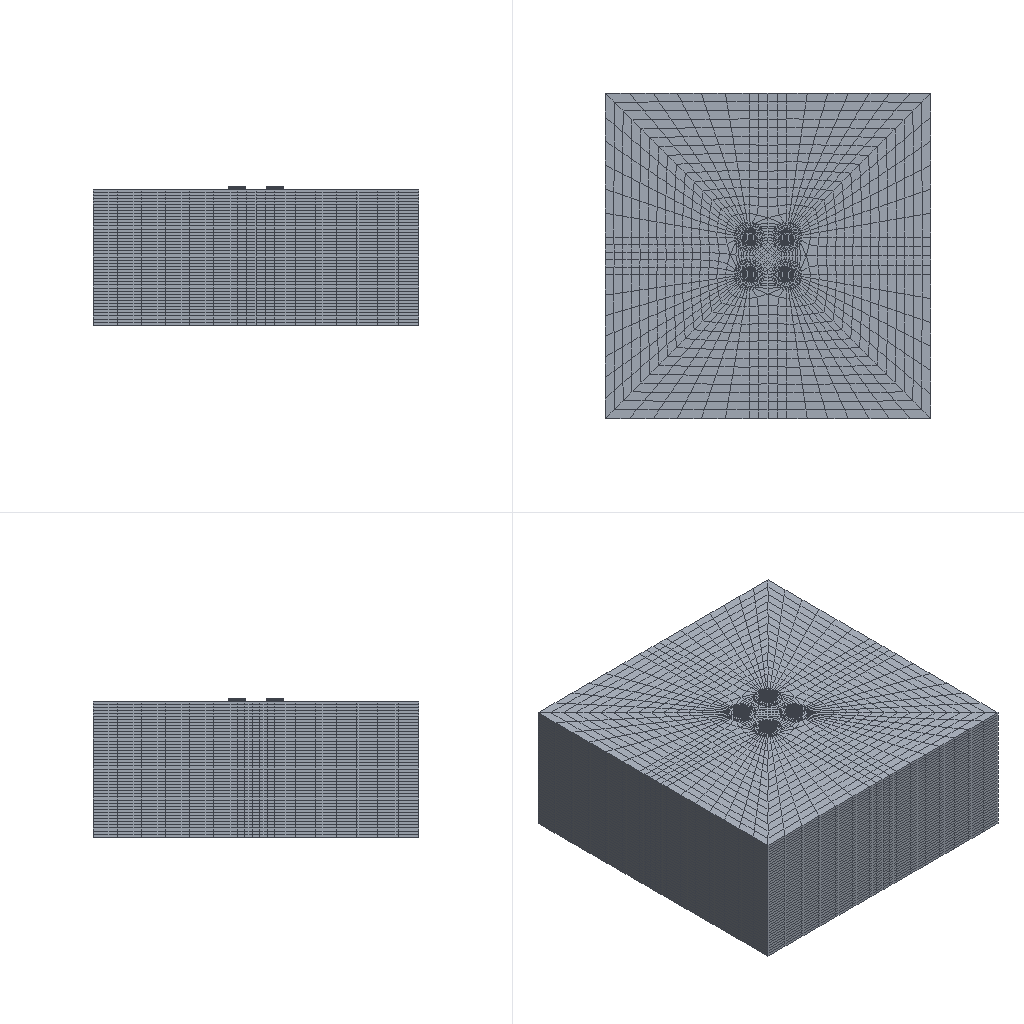Simulation study | abaqus
Set-up summary:
category,name,step,type,value,unit,region
solver,abaqus
solver,version,,,Abaqus/Standard 2020
units,not stated in the deck,,not stated
analysis,deck,,static,static
load_step,Step-digit-1,Step-digit-1,static
load_step,requested,,,1
mesh,nodes,,,107772
mesh,elements,,,93262
element_type,B31,,beam,40
element_type,C3D10,,solid,3792
element_type,C3D8R,,solid,89430
load,load commands in deck,,count,1
bc,support commands in deck,,count,3
material,TIE,,in results
material,TUTI,,in results
check,setup vs results,,match,"per instance, exact: element labels, types and connectivity; labels of the nodes the elements use; coordinates of those nodes at SINGLE_PRECISION in 8 of 21 instance(s)"
Abaqus input file, long lists of numbers shortened, first 379 of 1982 lines:
*Heading
** Job name: Job-1 Model name: Model-1
** Generated by: Abaqus/CAE 2020
*Preprint, echo=NO, model=NO, history=NO, contact=NO
**
** PARTS
**
*Part, name=chongshuatu
*Node
      1,           0., -0.0546, -0.1365
      2,           0.,           0., -0.1365
** (1960 more lines like these left out)
*Element, type=C3D10
  1, 321, 151,  35,  33, 350, 349, 348, 352, 351, 353
  2, 321, 152,  23,  34, 356, 355, 354, 358, 357, 359
** (946 more lines like these left out)
*Nset, nset=Set-chongshuatu, generate
    1,  1962,     1
*Elset, elset=Set-chongshuatu, generate
   1,  948,    1
** Section: Section-tuti
*Solid Section, elset=Set-chongshuatu, material=tuti
,
*End Part
**
*Part, name=daoguanzu
*Node
      1,           0.,           0.,           0.
      2,           0., 0.005,           0.
** (9 more lines like these left out)
*Element, type=B31
 1,  1,  2
 2,  2,  3
** (8 more lines like these left out)
*Nset, nset=Set-dgjzu, generate
  1,  11,   1
*Elset, elset=Set-dgjzu, generate
  1,  10,   1
** Section: Section-daoguanjia  Profile: Profile-dgj
*Beam Section, elset=Set-dgjzu, material=tie, temperature=GRADIENTS, section=CIRC
0.01
0.,0.,-1.
*End Part
**
*Part, name=tonggai
*Node
      1,  0.1365,           0.,           0.
      2,           0.,           0.,           0.
** (691 more lines like these left out)
*Element, type=C3D8R
  1, 194, 195, 545, 540,  15,  16, 149, 148
  2, 195, 196, 546, 545,  16,  17, 150, 149
** (414 more lines like these left out)
*Nset, nset=Set-tonggai, generate
   1,  693,    1
*Elset, elset=Set-tonggai, generate
   1,  416,    1
** Section: Section-tong
*Solid Section, elset=Set-tonggai, material=tie
,
*End Part
**
*Part, name=tongneitu
*Node
      1,  0.1265,           0.,           0.
      2,           0.,           0.,           0.
** (1307 more lines like these left out)
*Element, type=C3D8R
  1, 194, 195, 736, 680,  13,  14, 141, 140
  2, 195, 196, 737, 736,  14,  15, 142, 141
** (1038 more lines like these left out)
*Nset, nset=Set-tongneitu, generate
    1,  1309,     1
*Elset, elset=Set-tongneitu, generate
    1,  1040,     1
** Section: Section-tuti
*Solid Section, elset=Set-tongneitu, material=tuti
,
*End Part
**
*Part, name=tongqun
*Node
      1,           0.,  0.1265,  0.273
      2,           0.,  0.1265,           0.
** (2126 more lines like these left out)
*Element, type=C3D8R
  1,    8,  113,  752,  158,    1,    9,  293,   96
  2,  113,  112,  753,  752,    9,   10,  294,  293
** (1006 more lines like these left out)
*Nset, nset=Set-tongqun, generate
    1,  2128,     1
*Elset, elset=Set-tongqun, generate
    1,  1008,     1
** Section: Section-tong
*Solid Section, elset=Set-tongqun, material=tie
,
*End Part
**
*Part, name=tuti
*Node
      1,  -2.827,   2.417,  -2.184
      2,  -2.924,    2.32,  -2.184
** (83358 more lines like these left out)
*Element, type=C3D8R
  1,  4702,  4703, 33021, 32910,   204,   205,  4621,  4620
  2,  4703,  4704, 33022, 33021,   205,   206,  4622,  4621
** (79572 more lines like these left out)
*Nset, nset=Set-tuti, generate
     1,  83360,      1
*Elset, elset=Set-tuti, generate
     1,  79574,      1
** Section: Section-tuti
*Solid Section, elset=Set-tuti, material=tuti
,
*End Part
**
**
** ASSEMBLY
**
*Assembly, name=Assembly
**
*Instance, name=tonggai-1, part=tonggai
      0.3015,      -0.3015,         0.04
*End Instance
**
*Instance, name=tongneitu-1, part=tongneitu
      0.3015,      -0.3015,       -0.233
*End Instance
**
*Instance, name=tongqun-1, part=tongqun
      0.3015,      -0.3015,       -0.233
*End Instance
**
*Instance, name=tuti-1, part=tuti
       2.622,       -2.622,           0.
*End Instance
**
*Instance, name=tonggai-1-lin-1-2, part=tonggai
      0.3015,       0.3015,         0.04
*End Instance
**
*Instance, name=tonggai-1-lin-2-1, part=tonggai
     -0.3015,      -0.3015,         0.04
*End Instance
**
*Instance, name=tonggai-1-lin-2-2, part=tonggai
     -0.3015,       0.3015,         0.04
*End Instance
**
*Instance, name=tongneitu-1-lin-1-2, part=tongneitu
      0.3015,       0.3015,       -0.233
*End Instance
**
*Instance, name=tongneitu-1-lin-2-1, part=tongneitu
     -0.3015,      -0.3015,       -0.233
*End Instance
**
*Instance, name=tongneitu-1-lin-2-2, part=tongneitu
     -0.3015,       0.3015,       -0.233
*End Instance
**
*Instance, name=tongqun-1-lin-1-2, part=tongqun
      0.3015,       0.3015,       -0.233
*End Instance
**
*Instance, name=tongqun-1-lin-2-1, part=tongqun
     -0.3015,      -0.3015,       -0.233
*End Instance
**
*Instance, name=tongqun-1-lin-2-2, part=tongqun
     -0.3015,       0.3015,       -0.233
*End Instance
**
*Instance, name=chongshuatu-1, part=chongshuatu
      0.3015,      -0.3015,           0.
      0.3015,      -0.3015,           0., 1.302,      -0.3015,           0., 90.
*End Instance
**
*Instance, name=chongshuatu-1-lin-1-2, part=chongshuatu
      0.3015,       0.3015,           0.
      0.3015,       0.3015,           0., 1.302,       0.3015,           0., 90.
*End Instance
**
*Instance, name=chongshuatu-1-lin-2-1, part=chongshuatu
     -0.3015,      -0.3015,           0.
     -0.3015,      -0.3015,           0., 0.6985,      -0.3015,           0., 90.
*End Instance
**
*Instance, name=chongshuatu-1-lin-2-2, part=chongshuatu
     -0.3015,       0.3015,           0.
     -0.3015,       0.3015,           0., 0.6985,       0.3015,           0., 90.
*End Instance
**
*Instance, name=daoguanzu-1, part=daoguanzu
     -0.3015,      -0.3015,         0.05
     -0.3015,      -0.3015,         0.05, 0.6985,      -0.3015,         0.05, 90.
*End Instance
**
*Instance, name=daoguanzu-1-lin-1-2, part=daoguanzu
     -0.3015,       0.3015,         0.05
     -0.3015,       0.3015,         0.05, 0.6985,       0.3015,         0.05, 90.
*End Instance
**
*Instance, name=daoguanzu-1-lin-2-1, part=daoguanzu
0.3015,      -0.3015,         0.05
0.3015,      -0.3015,         0.05, 1.302,      -0.3015,         0.05, 90.
*End Instance
**
*Instance, name=daoguanzu-1-lin-2-2, part=daoguanzu
0.3015,       0.3015,         0.05
0.3015,       0.3015,         0.05, 1.302,       0.3015,         0.05, 90.
*End Instance
**
*Nset, nset=Set-10, instance=chongshuatu-1, generate
    1,  1962,     1
*Elset, elset=Set-10, instance=chongshuatu-1, generate
   1,  948,    1
*Nset, nset=Set-11, instance=chongshuatu-1-lin-1-2, generate
    1,  1962,     1
*Elset, elset=Set-11, instance=chongshuatu-1-lin-1-2, generate
   1,  948,    1
*Nset, nset=Set-12, instance=chongshuatu-1-lin-2-2, generate
    1,  1962,     1
*Elset, elset=Set-12, instance=chongshuatu-1-lin-2-2, generate
   1,  948,    1
*Nset, nset=Set-13, instance=chongshuatu-1-lin-2-1, generate
    1,  1962,     1
*Elset, elset=Set-13, instance=chongshuatu-1-lin-2-1, generate
   1,  948,    1
*Nset, nset=Set-14, instance=tuti-1
     1,     2,     3,    10,    11,    12,    25,    26,    27,    28,    31,    32,    35,    36,    44,    45
    46,    47,    48,    49,    50,    51,    52,    63,    64,    65,    81,    82,    83,    84,    88,    91
** (117 more lines like these left out)
*Elset, elset=Set-14, instance=tuti-1
     1,     2,     3,     4,     5,     6,   115,   116,   117,   172,   173,   734,   735,   774,   775,   814
   815,   873,   893,   913,   933,   953,   973,   974,   975,  1014,  1015,  5569,  5570,  5571,  5572,  5573
** (114 more lines like these left out)
*Nset, nset=Set-15, instance=tuti-1
    13,    16,    17,    20,    22,    25,    47,    48,    85,   113,   120,   141,   154,   155,   156,   157
   159,   160,   162,   163,   166,   167,   168,   183,   506,   507,   508,   509,   510,   511,   546,   547
** (100 more lines like these left out)
*Elset, elset=Set-15, instance=tuti-1
  1054,  1069,  1084,  1099,  1114,  1129,  1144,  1159,  1174,  1189,  1204,  1219,  1234,  1249,  1264,  1279
  1294,  1309,  1324,  1339,  1354,  1369,  1384,  1399,  1414,  1429,  1444,  1459,  1474,  1489,  1504,  1519
** (92 more lines like these left out)
*Nset, nset=Set-16, instance=tuti-1
    13,    17,    22,    23,    25,    26,    47,    85,    86,   113,   116,   119,   120,   141,   144,   154
   157,   159,   177,   178,   179,   198,   199,   202,   556,   557,   558,   559,   582,   583,   584,   585
** (100 more lines like these left out)
*Elset, elset=Set-16, instance=tuti-1
  1593,  1608,  1623,  1638,  1653,  1668,  1683,  1698,  1713,  1728,  1743,  1758,  1773,  1788,  1803,  1818
  1833,  1848,  1863,  1878,  1893,  1908,  1923,  1938,  1953,  1968,  1983,  1998,  2013,  2028,  2043,  2058
** (92 more lines like these left out)
*Nset, nset=Set-di, instance=tuti-1
     1,     2,     3,    10,    11,    12,    25,    26,    27,    28,    31,    32,    35,    36,    44,    45
    46,    47,    48,    49,    50,    51,    52,    63,    64,    65,    81,    82,    83,    84,    88,    91
** (117 more lines like these left out)
*Elset, elset=Set-di, instance=tuti-1
     1,     2,     3,     4,     5,     6,   115,   116,   117,   172,   173,   734,   735,   774,   775,   814
   815,   873,   893,   913,   933,   953,   973,   974,   975,  1014,  1015,  5569,  5570,  5571,  5572,  5573
** (114 more lines like these left out)
*Nset, nset=Set-shuiping, instance=tuti-1
    13,    16,    17,    20,    22,    23,    25,    26,    47,    48,    85,    86,   113,   116,   119,   120
   141,   144,   154,   155,   156,   157,   159,   160,   162,   163,   166,   167,   168,   177,   178,   179
** (190 more lines like these left out)
*Elset, elset=Set-shuiping, instance=tuti-1
  1054,  1069,  1084,  1099,  1114,  1129,  1144,  1159,  1174,  1189,  1204,  1219,  1234,  1249,  1264,  1279
  1294,  1309,  1324,  1339,  1354,  1369,  1384,  1399,  1414,  1429,  1444,  1459,  1474,  1489,  1504,  1519
** (185 more lines like these left out)
*Nset, nset=b_Set-5, instance=tonggai-1, generate
   1,  693,    1
*Nset, nset=b_Set-5, instance=tongqun-1, generate
    1,  2128,     1
*Nset, nset=b_Set-5, instance=tonggai-1-lin-1-2, generate
   1,  693,    1
*Nset, nset=b_Set-5, instance=tonggai-1-lin-2-2, generate
   1,  693,    1
*Nset, nset=b_Set-5, instance=tongqun-1-lin-1-2, generate
    1,  2128,     1
*Nset, nset=b_Set-5, instance=daoguanzu-1, generate
  1,  11,   1
*Nset, nset=b_Set-5, instance=tongqun-1-lin-2-2, generate
    1,  2128,     1
*Nset, nset=b_Set-5, instance=daoguanzu-1-lin-2-1, generate
  1,  11,   1
*Nset, nset=b_Set-5, instance=tonggai-1-lin-2-1, generate
   1,  693,    1
*Nset, nset=b_Set-5, instance=tongqun-1-lin-2-1, generate
    1,  2128,     1
*Nset, nset=b_Set-5, instance=daoguanzu-1-lin-1-2, generate
  1,  11,   1
*Nset, nset=b_Set-5, instance=daoguanzu-1-lin-2-2, generate
  1,  11,   1
*Elset, elset=b_Set-5, instance=tonggai-1, generate
   1,  416,    1
*Elset, elset=b_Set-5, instance=tongqun-1, generate
    1,  1008,     1
*Elset, elset=b_Set-5, instance=tonggai-1-lin-1-2, generate
   1,  416,    1
*Elset, elset=b_Set-5, instance=tonggai-1-lin-2-2, generate
   1,  416,    1
*Elset, elset=b_Set-5, instance=tongqun-1-lin-1-2, generate
    1,  1008,     1
*Elset, elset=b_Set-5, instance=daoguanzu-1, generate
  1,  10,   1
*Elset, elset=b_Set-5, instance=tongqun-1-lin-2-2, generate
    1,  1008,     1
*Elset, elset=b_Set-5, instance=daoguanzu-1-lin-2-1, generate
  1,  10,   1
*Elset, elset=b_Set-5, instance=tonggai-1-lin-2-1, generate
   1,  416,    1
*Elset, elset=b_Set-5, instance=tongqun-1-lin-2-1, generate
    1,  1008,     1
*Elset, elset=b_Set-5, instance=daoguanzu-1-lin-1-2, generate
  1,  10,   1
*Elset, elset=b_Set-5, instance=daoguanzu-1-lin-2-2, generate
  1,  10,   1
*Nset, nset=b_Set-6, instance=tonggai-1, generate
   1,  693,    1
*Nset, nset=b_Set-6, instance=tongqun-1, generate
    1,  2128,     1
*Nset, nset=b_Set-6, instance=tonggai-1-lin-1-2, generate
   1,  693,    1
*Nset, nset=b_Set-6, instance=tonggai-1-lin-2-2, generate
   1,  693,    1
*Nset, nset=b_Set-6, instance=tongqun-1-lin-1-2, generate
    1,  2128,     1
*Nset, nset=b_Set-6, instance=daoguanzu-1, generate
  1,  11,   1
*Nset, nset=b_Set-6, instance=tongqun-1-lin-2-2, generate
    1,  2128,     1
*Nset, nset=b_Set-6, instance=daoguanzu-1-lin-2-1, generate
  1,  11,   1
*Nset, nset=b_Set-6, instance=tonggai-1-lin-2-1, generate
   1,  693,    1
*Nset, nset=b_Set-6, instance=tongqun-1-lin-2-1, generate
    1,  2128,     1
*Nset, nset=b_Set-6, instance=daoguanzu-1-lin-1-2, generate
  1,  11,   1
*Nset, nset=b_Set-6, instance=daoguanzu-1-lin-2-2, generate
  1,  11,   1
*Elset, elset=b_Set-6, instance=tonggai-1, generate
   1,  416,    1
*Elset, elset=b_Set-6, instance=tongqun-1, generate
    1,  1008,     1
*Elset, elset=b_Set-6, instance=tonggai-1-lin-1-2, generate
   1,  416,    1
*Elset, elset=b_Set-6, instance=tonggai-1-lin-2-2, generate
   1,  416,    1
*Elset, elset=b_Set-6, instance=tongqun-1-lin-1-2, generate
    1,  1008,     1
*Elset, elset=b_Set-6, instance=daoguanzu-1, generate
  1,  10,   1
*Elset, elset=b_Set-6, instance=tongqun-1-lin-2-2, generate
    1,  1008,     1
*Elset, elset=b_Set-6, instance=daoguanzu-1-lin-2-1, generate
  1,  10,   1
*Elset, elset=b_Set-6, instance=tonggai-1-lin-2-1, generate
   1,  416,    1
*Elset, elset=b_Set-6, instance=tongqun-1-lin-2-1, generate
    1,  1008,     1
*Elset, elset=b_Set-6, instance=daoguanzu-1-lin-1-2, generate
  1,  10,   1
*Elset, elset=b_Set-6, instance=daoguanzu-1-lin-2-2, generate
  1,  10,   1
*Nset, nset=s_Set-zu1, instance=daoguanzu-1-lin-1-2
 1,
*Nset, nset=s_Set-zu2, instance=daoguanzu-1-lin-2-2
 1,
*Nset, nset=s_Set-zu3, instance=daoguanzu-1-lin-2-1
 1,
*Nset, nset=s_Set-zu4, instance=daoguanzu-1
 1,
*Elset, elset=_Surf-tongdi1_S6, internal, instance=tongqun-1-lin-2-2, generate
 505,  991,   18
*Elset, elset=_Surf-tongdi1_S4, internal, instance=tongqun-1-lin-2-2, generate
  18,  504,   18
*Surface, type=ELEMENT, name=Surf-tongdi1
_Surf-tongdi1_S6, S6
Last 618 lines:
*Surface, type=ELEMENT, name=_Int-1_gcs0_535, internal
__Int-1_gcs0_535_S3, S3
__Int-1_gcs0_535_S4, S4
*Elset, elset=__Int-1_gcs0_536_S4, internal, instance=tongneitu-1-lin-2-2
  842,  844,  846,  848,  850,  852,  854,  856,  858,  860,  862,  864,  866,  868,  870,  872
  874,  876,  878,  880,  912,  914,  916,  918,  920,  922,  924,  926,  928,  930,  932,  934
** (2 more lines like these left out)
*Elset, elset=__Int-1_gcs0_536_S3, internal, instance=tongneitu-1-lin-2-2
 881, 882, 883, 887, 888, 889, 893, 894, 895, 899, 900, 901, 905, 906, 907
*Surface, type=ELEMENT, name=_Int-1_gcs0_536, internal
__Int-1_gcs0_536_S4, S4
__Int-1_gcs0_536_S3, S3
*Elset, elset=__Int-1_gcs0_542_S1, internal, instance=tongqun-1-lin-1-2, generate
  505,  1008,     1
*Surface, type=ELEMENT, name=_Int-1_gcs0_542, internal
__Int-1_gcs0_542_S1, S1
*Elset, elset=__Int-1_gcs0_544_S2, internal, instance=tongqun-1-lin-1-2, generate
   1,  504,    1
*Surface, type=ELEMENT, name=_Int-1_gcs0_544, internal
__Int-1_gcs0_544_S2, S2
*Elset, elset=__Int-1_gcs0_545_S1, internal, instance=tongqun-1-lin-1-2, generate
   1,  504,    1
*Surface, type=ELEMENT, name=_Int-1_gcs0_545, internal
__Int-1_gcs0_545_S1, S1
*Elset, elset=__Int-1_gcs0_546_S2, internal, instance=tongqun-1-lin-1-2, generate
  505,  1008,     1
*Surface, type=ELEMENT, name=_Int-1_gcs0_546, internal
__Int-1_gcs0_546_S2, S2
*Elset, elset=__Int-1_gcs0_552_S1, internal, instance=tongqun-1-lin-2-1, generate
  505,  1008,     1
*Surface, type=ELEMENT, name=_Int-1_gcs0_552, internal
__Int-1_gcs0_552_S1, S1
*Elset, elset=__Int-1_gcs0_554_S2, internal, instance=tongqun-1-lin-2-1, generate
   1,  504,    1
*Surface, type=ELEMENT, name=_Int-1_gcs0_554, internal
__Int-1_gcs0_554_S2, S2
*Elset, elset=__Int-1_gcs0_555_S1, internal, instance=tongqun-1-lin-2-1, generate
   1,  504,    1
*Surface, type=ELEMENT, name=_Int-1_gcs0_555, internal
__Int-1_gcs0_555_S1, S1
*Elset, elset=__Int-1_gcs0_556_S2, internal, instance=tongqun-1-lin-2-1, generate
  505,  1008,     1
*Surface, type=ELEMENT, name=_Int-1_gcs0_556, internal
__Int-1_gcs0_556_S2, S2
*Elset, elset=__Int-1_gcs0_562_S1, internal, instance=tongqun-1-lin-2-2, generate
  505,  1008,     1
*Surface, type=ELEMENT, name=_Int-1_gcs0_562, internal
__Int-1_gcs0_562_S1, S1
*Elset, elset=__Int-1_gcs0_564_S2, internal, instance=tongqun-1-lin-2-2, generate
   1,  504,    1
*Surface, type=ELEMENT, name=_Int-1_gcs0_564, internal
__Int-1_gcs0_564_S2, S2
*Elset, elset=__Int-1_gcs0_565_S1, internal, instance=tongqun-1-lin-2-2, generate
   1,  504,    1
*Surface, type=ELEMENT, name=_Int-1_gcs0_565, internal
__Int-1_gcs0_565_S1, S1
*Elset, elset=__Int-1_gcs0_566_S2, internal, instance=tongqun-1-lin-2-2, generate
  505,  1008,     1
*Surface, type=ELEMENT, name=_Int-1_gcs0_566, internal
__Int-1_gcs0_566_S2, S2
*Elset, elset=__Int-1_gcs0_572_S3, internal, instance=chongshuatu-1
  16,  23,  45,  51,  72,  80,  84,  96,  98,  99, 101, 102, 106, 111, 116, 130
 134, 139, 141, 142, 145, 149, 165, 173, 178, 183, 190, 194, 218, 243
*Elset, elset=__Int-1_gcs0_572_S4, internal, instance=chongshuatu-1
  33,  90, 112, 120, 132, 174, 175, 185, 209, 213, 216, 226
*Elset, elset=__Int-1_gcs0_572_S1, internal, instance=chongshuatu-1
  78,  83,  95, 128, 136, 147, 168, 179, 182, 187, 204, 206, 210, 228, 233, 240
 242,
*Elset, elset=__Int-1_gcs0_572_S2, internal, instance=chongshuatu-1
  81,  89, 191, 207, 238
*Surface, type=ELEMENT, name=_Int-1_gcs0_572, internal
__Int-1_gcs0_572_S3, S3
__Int-1_gcs0_572_S4, S4
__Int-1_gcs0_572_S2, S2
__Int-1_gcs0_572_S1, S1
*Elset, elset=__Int-1_gcs0_573_S3, internal, instance=chongshuatu-1
  61, 148, 153, 160, 169, 170, 171, 172, 175, 179, 180, 181, 182, 184, 187, 188
 189, 191, 192, 193, 199, 200, 203, 205, 207, 210, 211, 217, 238
*Elset, elset=__Int-1_gcs0_573_S1, internal, instance=chongshuatu-1
  94, 151
*Elset, elset=__Int-1_gcs0_573_S2, internal, instance=chongshuatu-1
 186,
*Surface, type=ELEMENT, name=_Int-1_gcs0_573, internal
__Int-1_gcs0_573_S3, S3
__Int-1_gcs0_573_S1, S1
__Int-1_gcs0_573_S2, S2
*Elset, elset=__Int-1_gcs0_574_S3, internal, instance=chongshuatu-1
 534, 543, 593, 634, 642, 645, 652, 658, 661, 662, 670, 674, 675, 676, 680, 681
 682, 685, 690, 692, 694, 697, 698, 703, 706, 707, 708, 716, 718, 727
*Elset, elset=__Int-1_gcs0_574_S2, internal, instance=chongshuatu-1
 663,
*Elset, elset=__Int-1_gcs0_574_S4, internal, instance=chongshuatu-1
 664,
*Surface, type=ELEMENT, name=_Int-1_gcs0_574, internal
__Int-1_gcs0_574_S3, S3
__Int-1_gcs0_574_S2, S2
__Int-1_gcs0_574_S4, S4
*Elset, elset=__Int-1_gcs0_575_S3, internal, instance=chongshuatu-1
 252, 283, 306, 312, 315, 321, 337, 363, 366, 367, 374, 389, 416, 429, 434, 444
 458, 465, 469, 479
*Elset, elset=__Int-1_gcs0_575_S2, internal, instance=chongshuatu-1
 269, 314, 328, 377, 384, 412, 446, 448
*Elset, elset=__Int-1_gcs0_575_S1, internal, instance=chongshuatu-1
 308, 309, 313, 318, 323, 332, 339, 342, 346, 347, 348, 378, 380, 400, 415, 420
 431, 450, 453, 466, 489
*Elset, elset=__Int-1_gcs0_575_S4, internal, instance=chongshuatu-1
 310, 311, 319, 331, 344, 355, 357, 358, 361, 369, 371, 382, 394, 402, 433
*Surface, type=ELEMENT, name=_Int-1_gcs0_575, internal
__Int-1_gcs0_575_S3, S3
__Int-1_gcs0_575_S2, S2
__Int-1_gcs0_575_S4, S4
__Int-1_gcs0_575_S1, S1
*Elset, elset=__Int-1_gcs0_580_S3, internal, instance=chongshuatu-1
 507, 511, 530, 541, 548, 555, 557, 561, 578, 579, 580, 589, 594, 603, 604, 606
 613, 617, 626, 641, 643, 647, 648, 656, 671, 672, 684, 735
*Elset, elset=__Int-1_gcs0_580_S2, internal, instance=chongshuatu-1
 516, 629, 639, 716, 727
*Elset, elset=__Int-1_gcs0_580_S1, internal, instance=chongshuatu-1
 517, 534, 611, 624, 636, 640, 644, 663, 668, 675, 676, 686, 703, 704, 709, 728
*Elset, elset=__Int-1_gcs0_580_S4, internal, instance=chongshuatu-1
 522, 529, 552, 592, 595, 599, 610, 631, 645, 666, 673, 677, 679, 714, 732
*Surface, type=ELEMENT, name=_Int-1_gcs0_580, internal
__Int-1_gcs0_580_S3, S3
__Int-1_gcs0_580_S2, S2
__Int-1_gcs0_580_S4, S4
__Int-1_gcs0_580_S1, S1
*Elset, elset=__Int-1_gcs0_581_S3, internal, instance=chongshuatu-1
 246, 259, 264, 278, 286, 292, 296, 302, 311, 314, 332, 360, 379, 423, 441, 448
 452, 454, 466, 473, 488, 489
*Elset, elset=__Int-1_gcs0_581_S2, internal, instance=chongshuatu-1
 304, 486
*Elset, elset=__Int-1_gcs0_581_S1, internal, instance=chongshuatu-1
 324, 375, 376, 469, 476, 480, 484
*Elset, elset=__Int-1_gcs0_581_S4, internal, instance=chongshuatu-1
 465,
*Surface, type=ELEMENT, name=_Int-1_gcs0_581, internal
__Int-1_gcs0_581_S3, S3
__Int-1_gcs0_581_S2, S2
__Int-1_gcs0_581_S4, S4
__Int-1_gcs0_581_S1, S1
*Elset, elset=__Int-1_gcs0_582_S3, internal, instance=chongshuatu-1
 737, 738, 746, 756, 758
*Elset, elset=__Int-1_gcs0_582_S4, internal, instance=chongshuatu-1
 745, 786, 869, 880, 892, 902, 911, 938, 943, 947
*Elset, elset=__Int-1_gcs0_582_S1, internal, instance=chongshuatu-1
 771, 776, 777, 791, 847, 873, 891, 912, 914, 939, 946, 948
*Elset, elset=__Int-1_gcs0_582_S2, internal, instance=chongshuatu-1
 850, 860, 870, 934, 944
*Surface, type=ELEMENT, name=_Int-1_gcs0_582, internal
__Int-1_gcs0_582_S3, S3
__Int-1_gcs0_582_S4, S4
__Int-1_gcs0_582_S2, S2
__Int-1_gcs0_582_S1, S1
*Elset, elset=__Int-1_gcs0_583_S3, internal, instance=chongshuatu-1
 740, 751, 752, 761, 777, 798, 801, 820, 833, 852, 859, 860, 861, 869, 873, 885
 891, 909, 912, 917, 934, 938
*Elset, elset=__Int-1_gcs0_583_S1, internal, instance=chongshuatu-1
 759, 760, 774, 775, 785, 810, 824, 843, 899
*Elset, elset=__Int-1_gcs0_583_S2, internal, instance=chongshuatu-1
 768, 772, 779, 780, 781, 792, 793, 796, 797, 799, 803, 804, 805, 806, 811, 818
 823, 826, 837, 854, 877, 886, 894, 904, 924, 926, 933
*Elset, elset=__Int-1_gcs0_583_S4, internal, instance=chongshuatu-1
 769, 808, 816, 835, 883, 927
*Surface, type=ELEMENT, name=_Int-1_gcs0_583, internal
__Int-1_gcs0_583_S3, S3
__Int-1_gcs0_583_S1, S1
__Int-1_gcs0_583_S2, S2
__Int-1_gcs0_583_S4, S4
*Elset, elset=__Int-1_gcs0_588_S3, internal, instance=chongshuatu-1-lin-1-2
  16,  23,  45,  51,  72,  80,  84,  96,  98,  99, 101, 102, 106, 111, 116, 130
 134, 139, 141, 142, 145, 149, 165, 173, 178, 183, 190, 194, 218, 243
*Elset, elset=__Int-1_gcs0_588_S4, internal, instance=chongshuatu-1-lin-1-2
  33,  90, 112, 120, 132, 174, 175, 185, 209, 213, 216, 226
*Elset, elset=__Int-1_gcs0_588_S1, internal, instance=chongshuatu-1-lin-1-2
  78,  83,  95, 128, 136, 147, 168, 179, 182, 187, 204, 206, 210, 228, 233, 240
 242,
*Elset, elset=__Int-1_gcs0_588_S2, internal, instance=chongshuatu-1-lin-1-2
  81,  89, 191, 207, 238
*Surface, type=ELEMENT, name=_Int-1_gcs0_588, internal
__Int-1_gcs0_588_S3, S3
__Int-1_gcs0_588_S4, S4
__Int-1_gcs0_588_S2, S2
__Int-1_gcs0_588_S1, S1
*Elset, elset=__Int-1_gcs0_589_S3, internal, instance=chongshuatu-1-lin-1-2
  61, 148, 153, 160, 169, 170, 171, 172, 175, 179, 180, 181, 182, 184, 187, 188
 189, 191, 192, 193, 199, 200, 203, 205, 207, 210, 211, 217, 238
*Elset, elset=__Int-1_gcs0_589_S1, internal, instance=chongshuatu-1-lin-1-2
  94, 151
*Elset, elset=__Int-1_gcs0_589_S2, internal, instance=chongshuatu-1-lin-1-2
 186,
*Surface, type=ELEMENT, name=_Int-1_gcs0_589, internal
__Int-1_gcs0_589_S3, S3
__Int-1_gcs0_589_S1, S1
__Int-1_gcs0_589_S2, S2
*Elset, elset=__Int-1_gcs0_590_S3, internal, instance=chongshuatu-1-lin-1-2
 534, 543, 593, 634, 642, 645, 652, 658, 661, 662, 670, 674, 675, 676, 680, 681
 682, 685, 690, 692, 694, 697, 698, 703, 706, 707, 708, 716, 718, 727
*Elset, elset=__Int-1_gcs0_590_S2, internal, instance=chongshuatu-1-lin-1-2
 663,
*Elset, elset=__Int-1_gcs0_590_S4, internal, instance=chongshuatu-1-lin-1-2
 664,
*Surface, type=ELEMENT, name=_Int-1_gcs0_590, internal
__Int-1_gcs0_590_S3, S3
__Int-1_gcs0_590_S2, S2
__Int-1_gcs0_590_S4, S4
*Elset, elset=__Int-1_gcs0_591_S3, internal, instance=chongshuatu-1-lin-1-2
 252, 283, 306, 312, 315, 321, 337, 363, 366, 367, 374, 389, 416, 429, 434, 444
 458, 465, 469, 479
*Elset, elset=__Int-1_gcs0_591_S2, internal, instance=chongshuatu-1-lin-1-2
 269, 314, 328, 377, 384, 412, 446, 448
*Elset, elset=__Int-1_gcs0_591_S1, internal, instance=chongshuatu-1-lin-1-2
 308, 309, 313, 318, 323, 332, 339, 342, 346, 347, 348, 378, 380, 400, 415, 420
 431, 450, 453, 466, 489
*Elset, elset=__Int-1_gcs0_591_S4, internal, instance=chongshuatu-1-lin-1-2
 310, 311, 319, 331, 344, 355, 357, 358, 361, 369, 371, 382, 394, 402, 433
*Surface, type=ELEMENT, name=_Int-1_gcs0_591, internal
__Int-1_gcs0_591_S3, S3
__Int-1_gcs0_591_S2, S2
__Int-1_gcs0_591_S4, S4
__Int-1_gcs0_591_S1, S1
*Elset, elset=__Int-1_gcs0_596_S3, internal, instance=chongshuatu-1-lin-1-2
 507, 511, 530, 541, 548, 555, 557, 561, 578, 579, 580, 589, 594, 603, 604, 606
 613, 617, 626, 641, 643, 647, 648, 656, 671, 672, 684, 735
*Elset, elset=__Int-1_gcs0_596_S2, internal, instance=chongshuatu-1-lin-1-2
 516, 629, 639, 716, 727
*Elset, elset=__Int-1_gcs0_596_S1, internal, instance=chongshuatu-1-lin-1-2
 517, 534, 611, 624, 636, 640, 644, 663, 668, 675, 676, 686, 703, 704, 709, 728
*Elset, elset=__Int-1_gcs0_596_S4, internal, instance=chongshuatu-1-lin-1-2
 522, 529, 552, 592, 595, 599, 610, 631, 645, 666, 673, 677, 679, 714, 732
*Surface, type=ELEMENT, name=_Int-1_gcs0_596, internal
__Int-1_gcs0_596_S3, S3
__Int-1_gcs0_596_S2, S2
__Int-1_gcs0_596_S4, S4
__Int-1_gcs0_596_S1, S1
*Elset, elset=__Int-1_gcs0_597_S3, internal, instance=chongshuatu-1-lin-1-2
 246, 259, 264, 278, 286, 292, 296, 302, 311, 314, 332, 360, 379, 423, 441, 448
 452, 454, 466, 473, 488, 489
*Elset, elset=__Int-1_gcs0_597_S2, internal, instance=chongshuatu-1-lin-1-2
 304, 486
*Elset, elset=__Int-1_gcs0_597_S1, internal, instance=chongshuatu-1-lin-1-2
 324, 375, 376, 469, 476, 480, 484
*Elset, elset=__Int-1_gcs0_597_S4, internal, instance=chongshuatu-1-lin-1-2
 465,
*Surface, type=ELEMENT, name=_Int-1_gcs0_597, internal
__Int-1_gcs0_597_S3, S3
__Int-1_gcs0_597_S2, S2
__Int-1_gcs0_597_S4, S4
__Int-1_gcs0_597_S1, S1
*Elset, elset=__Int-1_gcs0_598_S3, internal, instance=chongshuatu-1-lin-1-2
 737, 738, 746, 756, 758
*Elset, elset=__Int-1_gcs0_598_S4, internal, instance=chongshuatu-1-lin-1-2
 745, 786, 869, 880, 892, 902, 911, 938, 943, 947
*Elset, elset=__Int-1_gcs0_598_S1, internal, instance=chongshuatu-1-lin-1-2
 771, 776, 777, 791, 847, 873, 891, 912, 914, 939, 946, 948
*Elset, elset=__Int-1_gcs0_598_S2, internal, instance=chongshuatu-1-lin-1-2
 850, 860, 870, 934, 944
*Surface, type=ELEMENT, name=_Int-1_gcs0_598, internal
__Int-1_gcs0_598_S3, S3
__Int-1_gcs0_598_S4, S4
__Int-1_gcs0_598_S2, S2
__Int-1_gcs0_598_S1, S1
*Elset, elset=__Int-1_gcs0_599_S3, internal, instance=chongshuatu-1-lin-1-2
 740, 751, 752, 761, 777, 798, 801, 820, 833, 852, 859, 860, 861, 869, 873, 885
 891, 909, 912, 917, 934, 938
*Elset, elset=__Int-1_gcs0_599_S1, internal, instance=chongshuatu-1-lin-1-2
 759, 760, 774, 775, 785, 810, 824, 843, 899
*Elset, elset=__Int-1_gcs0_599_S2, internal, instance=chongshuatu-1-lin-1-2
 768, 772, 779, 780, 781, 792, 793, 796, 797, 799, 803, 804, 805, 806, 811, 818
 823, 826, 837, 854, 877, 886, 894, 904, 924, 926, 933
*Elset, elset=__Int-1_gcs0_599_S4, internal, instance=chongshuatu-1-lin-1-2
 769, 808, 816, 835, 883, 927
*Surface, type=ELEMENT, name=_Int-1_gcs0_599, internal
__Int-1_gcs0_599_S3, S3
__Int-1_gcs0_599_S1, S1
__Int-1_gcs0_599_S2, S2
__Int-1_gcs0_599_S4, S4
*Elset, elset=__Int-1_gcs0_604_S3, internal, instance=chongshuatu-1-lin-2-1
  16,  23,  45,  51,  72,  80,  84,  96,  98,  99, 101, 102, 106, 111, 116, 130
 134, 139, 141, 142, 145, 149, 165, 173, 178, 183, 190, 194, 218, 243
*Elset, elset=__Int-1_gcs0_604_S4, internal, instance=chongshuatu-1-lin-2-1
  33,  90, 112, 120, 132, 174, 175, 185, 209, 213, 216, 226
*Elset, elset=__Int-1_gcs0_604_S1, internal, instance=chongshuatu-1-lin-2-1
  78,  83,  95, 128, 136, 147, 168, 179, 182, 187, 204, 206, 210, 228, 233, 240
 242,
*Elset, elset=__Int-1_gcs0_604_S2, internal, instance=chongshuatu-1-lin-2-1
  81,  89, 191, 207, 238
*Surface, type=ELEMENT, name=_Int-1_gcs0_604, internal
__Int-1_gcs0_604_S3, S3
__Int-1_gcs0_604_S4, S4
__Int-1_gcs0_604_S2, S2
__Int-1_gcs0_604_S1, S1
*Elset, elset=__Int-1_gcs0_605_S3, internal, instance=chongshuatu-1-lin-2-1
  61, 148, 153, 160, 169, 170, 171, 172, 175, 179, 180, 181, 182, 184, 187, 188
 189, 191, 192, 193, 199, 200, 203, 205, 207, 210, 211, 217, 238
*Elset, elset=__Int-1_gcs0_605_S1, internal, instance=chongshuatu-1-lin-2-1
  94, 151
*Elset, elset=__Int-1_gcs0_605_S2, internal, instance=chongshuatu-1-lin-2-1
 186,
*Surface, type=ELEMENT, name=_Int-1_gcs0_605, internal
__Int-1_gcs0_605_S3, S3
__Int-1_gcs0_605_S1, S1
__Int-1_gcs0_605_S2, S2
*Elset, elset=__Int-1_gcs0_606_S3, internal, instance=chongshuatu-1-lin-2-1
 534, 543, 593, 634, 642, 645, 652, 658, 661, 662, 670, 674, 675, 676, 680, 681
 682, 685, 690, 692, 694, 697, 698, 703, 706, 707, 708, 716, 718, 727
*Elset, elset=__Int-1_gcs0_606_S2, internal, instance=chongshuatu-1-lin-2-1
 663,
*Elset, elset=__Int-1_gcs0_606_S4, internal, instance=chongshuatu-1-lin-2-1
 664,
*Surface, type=ELEMENT, name=_Int-1_gcs0_606, internal
__Int-1_gcs0_606_S3, S3
__Int-1_gcs0_606_S2, S2
__Int-1_gcs0_606_S4, S4
*Elset, elset=__Int-1_gcs0_607_S3, internal, instance=chongshuatu-1-lin-2-1
 252, 283, 306, 312, 315, 321, 337, 363, 366, 367, 374, 389, 416, 429, 434, 444
 458, 465, 469, 479
*Elset, elset=__Int-1_gcs0_607_S2, internal, instance=chongshuatu-1-lin-2-1
 269, 314, 328, 377, 384, 412, 446, 448
*Elset, elset=__Int-1_gcs0_607_S1, internal, instance=chongshuatu-1-lin-2-1
 308, 309, 313, 318, 323, 332, 339, 342, 346, 347, 348, 378, 380, 400, 415, 420
 431, 450, 453, 466, 489
*Elset, elset=__Int-1_gcs0_607_S4, internal, instance=chongshuatu-1-lin-2-1
 310, 311, 319, 331, 344, 355, 357, 358, 361, 369, 371, 382, 394, 402, 433
*Surface, type=ELEMENT, name=_Int-1_gcs0_607, internal
__Int-1_gcs0_607_S3, S3
__Int-1_gcs0_607_S2, S2
__Int-1_gcs0_607_S4, S4
__Int-1_gcs0_607_S1, S1
*Elset, elset=__Int-1_gcs0_612_S3, internal, instance=chongshuatu-1-lin-2-1
 507, 511, 530, 541, 548, 555, 557, 561, 578, 579, 580, 589, 594, 603, 604, 606
 613, 617, 626, 641, 643, 647, 648, 656, 671, 672, 684, 735
*Elset, elset=__Int-1_gcs0_612_S2, internal, instance=chongshuatu-1-lin-2-1
 516, 629, 639, 716, 727
*Elset, elset=__Int-1_gcs0_612_S1, internal, instance=chongshuatu-1-lin-2-1
 517, 534, 611, 624, 636, 640, 644, 663, 668, 675, 676, 686, 703, 704, 709, 728
*Elset, elset=__Int-1_gcs0_612_S4, internal, instance=chongshuatu-1-lin-2-1
 522, 529, 552, 592, 595, 599, 610, 631, 645, 666, 673, 677, 679, 714, 732
*Surface, type=ELEMENT, name=_Int-1_gcs0_612, internal
__Int-1_gcs0_612_S3, S3
__Int-1_gcs0_612_S2, S2
__Int-1_gcs0_612_S4, S4
__Int-1_gcs0_612_S1, S1
*Elset, elset=__Int-1_gcs0_613_S3, internal, instance=chongshuatu-1-lin-2-1
 246, 259, 264, 278, 286, 292, 296, 302, 311, 314, 332, 360, 379, 423, 441, 448
 452, 454, 466, 473, 488, 489
*Elset, elset=__Int-1_gcs0_613_S2, internal, instance=chongshuatu-1-lin-2-1
 304, 486
*Elset, elset=__Int-1_gcs0_613_S1, internal, instance=chongshuatu-1-lin-2-1
 324, 375, 376, 469, 476, 480, 484
*Elset, elset=__Int-1_gcs0_613_S4, internal, instance=chongshuatu-1-lin-2-1
 465,
*Surface, type=ELEMENT, name=_Int-1_gcs0_613, internal
__Int-1_gcs0_613_S3, S3
__Int-1_gcs0_613_S2, S2
__Int-1_gcs0_613_S4, S4
__Int-1_gcs0_613_S1, S1
*Elset, elset=__Int-1_gcs0_614_S3, internal, instance=chongshuatu-1-lin-2-1
 737, 738, 746, 756, 758
*Elset, elset=__Int-1_gcs0_614_S4, internal, instance=chongshuatu-1-lin-2-1
 745, 786, 869, 880, 892, 902, 911, 938, 943, 947
*Elset, elset=__Int-1_gcs0_614_S1, internal, instance=chongshuatu-1-lin-2-1
 771, 776, 777, 791, 847, 873, 891, 912, 914, 939, 946, 948
*Elset, elset=__Int-1_gcs0_614_S2, internal, instance=chongshuatu-1-lin-2-1
 850, 860, 870, 934, 944
*Surface, type=ELEMENT, name=_Int-1_gcs0_614, internal
__Int-1_gcs0_614_S3, S3
__Int-1_gcs0_614_S4, S4
__Int-1_gcs0_614_S2, S2
__Int-1_gcs0_614_S1, S1
*Elset, elset=__Int-1_gcs0_615_S3, internal, instance=chongshuatu-1-lin-2-1
 740, 751, 752, 761, 777, 798, 801, 820, 833, 852, 859, 860, 861, 869, 873, 885
 891, 909, 912, 917, 934, 938
*Elset, elset=__Int-1_gcs0_615_S1, internal, instance=chongshuatu-1-lin-2-1
 759, 760, 774, 775, 785, 810, 824, 843, 899
*Elset, elset=__Int-1_gcs0_615_S2, internal, instance=chongshuatu-1-lin-2-1
 768, 772, 779, 780, 781, 792, 793, 796, 797, 799, 803, 804, 805, 806, 811, 818
 823, 826, 837, 854, 877, 886, 894, 904, 924, 926, 933
*Elset, elset=__Int-1_gcs0_615_S4, internal, instance=chongshuatu-1-lin-2-1
 769, 808, 816, 835, 883, 927
*Surface, type=ELEMENT, name=_Int-1_gcs0_615, internal
__Int-1_gcs0_615_S3, S3
__Int-1_gcs0_615_S1, S1
__Int-1_gcs0_615_S2, S2
__Int-1_gcs0_615_S4, S4
*Elset, elset=__Int-1_gcs0_620_S3, internal, instance=chongshuatu-1-lin-2-2
  16,  23,  45,  51,  72,  80,  84,  96,  98,  99, 101, 102, 106, 111, 116, 130
 134, 139, 141, 142, 145, 149, 165, 173, 178, 183, 190, 194, 218, 243
*Elset, elset=__Int-1_gcs0_620_S4, internal, instance=chongshuatu-1-lin-2-2
  33,  90, 112, 120, 132, 174, 175, 185, 209, 213, 216, 226
*Elset, elset=__Int-1_gcs0_620_S1, internal, instance=chongshuatu-1-lin-2-2
  78,  83,  95, 128, 136, 147, 168, 179, 182, 187, 204, 206, 210, 228, 233, 240
 242,
*Elset, elset=__Int-1_gcs0_620_S2, internal, instance=chongshuatu-1-lin-2-2
  81,  89, 191, 207, 238
*Surface, type=ELEMENT, name=_Int-1_gcs0_620, internal
__Int-1_gcs0_620_S3, S3
__Int-1_gcs0_620_S4, S4
__Int-1_gcs0_620_S2, S2
__Int-1_gcs0_620_S1, S1
*Elset, elset=__Int-1_gcs0_621_S3, internal, instance=chongshuatu-1-lin-2-2
  61, 148, 153, 160, 169, 170, 171, 172, 175, 179, 180, 181, 182, 184, 187, 188
 189, 191, 192, 193, 199, 200, 203, 205, 207, 210, 211, 217, 238
*Elset, elset=__Int-1_gcs0_621_S1, internal, instance=chongshuatu-1-lin-2-2
  94, 151
*Elset, elset=__Int-1_gcs0_621_S2, internal, instance=chongshuatu-1-lin-2-2
 186,
*Surface, type=ELEMENT, name=_Int-1_gcs0_621, internal
__Int-1_gcs0_621_S3, S3
__Int-1_gcs0_621_S1, S1
__Int-1_gcs0_621_S2, S2
*Elset, elset=__Int-1_gcs0_622_S3, internal, instance=chongshuatu-1-lin-2-2
 534, 543, 593, 634, 642, 645, 652, 658, 661, 662, 670, 674, 675, 676, 680, 681
 682, 685, 690, 692, 694, 697, 698, 703, 706, 707, 708, 716, 718, 727
*Elset, elset=__Int-1_gcs0_622_S2, internal, instance=chongshuatu-1-lin-2-2
 663,
*Elset, elset=__Int-1_gcs0_622_S4, internal, instance=chongshuatu-1-lin-2-2
 664,
*Surface, type=ELEMENT, name=_Int-1_gcs0_622, internal
__Int-1_gcs0_622_S3, S3
__Int-1_gcs0_622_S2, S2
__Int-1_gcs0_622_S4, S4
*Elset, elset=__Int-1_gcs0_623_S3, internal, instance=chongshuatu-1-lin-2-2
 252, 283, 306, 312, 315, 321, 337, 363, 366, 367, 374, 389, 416, 429, 434, 444
 458, 465, 469, 479
*Elset, elset=__Int-1_gcs0_623_S2, internal, instance=chongshuatu-1-lin-2-2
 269, 314, 328, 377, 384, 412, 446, 448
*Elset, elset=__Int-1_gcs0_623_S1, internal, instance=chongshuatu-1-lin-2-2
 308, 309, 313, 318, 323, 332, 339, 342, 346, 347, 348, 378, 380, 400, 415, 420
 431, 450, 453, 466, 489
*Elset, elset=__Int-1_gcs0_623_S4, internal, instance=chongshuatu-1-lin-2-2
 310, 311, 319, 331, 344, 355, 357, 358, 361, 369, 371, 382, 394, 402, 433
*Surface, type=ELEMENT, name=_Int-1_gcs0_623, internal
__Int-1_gcs0_623_S3, S3
__Int-1_gcs0_623_S2, S2
__Int-1_gcs0_623_S4, S4
__Int-1_gcs0_623_S1, S1
*Elset, elset=__Int-1_gcs0_628_S3, internal, instance=chongshuatu-1-lin-2-2
 507, 511, 530, 541, 548, 555, 557, 561, 578, 579, 580, 589, 594, 603, 604, 606
 613, 617, 626, 641, 643, 647, 648, 656, 671, 672, 684, 735
*Elset, elset=__Int-1_gcs0_628_S2, internal, instance=chongshuatu-1-lin-2-2
 516, 629, 639, 716, 727
*Elset, elset=__Int-1_gcs0_628_S1, internal, instance=chongshuatu-1-lin-2-2
 517, 534, 611, 624, 636, 640, 644, 663, 668, 675, 676, 686, 703, 704, 709, 728
*Elset, elset=__Int-1_gcs0_628_S4, internal, instance=chongshuatu-1-lin-2-2
 522, 529, 552, 592, 595, 599, 610, 631, 645, 666, 673, 677, 679, 714, 732
*Surface, type=ELEMENT, name=_Int-1_gcs0_628, internal
__Int-1_gcs0_628_S3, S3
__Int-1_gcs0_628_S2, S2
__Int-1_gcs0_628_S4, S4
__Int-1_gcs0_628_S1, S1
*Elset, elset=__Int-1_gcs0_629_S3, internal, instance=chongshuatu-1-lin-2-2
 246, 259, 264, 278, 286, 292, 296, 302, 311, 314, 332, 360, 379, 423, 441, 448
 452, 454, 466, 473, 488, 489
*Elset, elset=__Int-1_gcs0_629_S2, internal, instance=chongshuatu-1-lin-2-2
 304, 486
*Elset, elset=__Int-1_gcs0_629_S1, internal, instance=chongshuatu-1-lin-2-2
 324, 375, 376, 469, 476, 480, 484
*Elset, elset=__Int-1_gcs0_629_S4, internal, instance=chongshuatu-1-lin-2-2
 465,
*Surface, type=ELEMENT, name=_Int-1_gcs0_629, internal
__Int-1_gcs0_629_S3, S3
__Int-1_gcs0_629_S2, S2
__Int-1_gcs0_629_S4, S4
__Int-1_gcs0_629_S1, S1
*Elset, elset=__Int-1_gcs0_630_S3, internal, instance=chongshuatu-1-lin-2-2
 737, 738, 746, 756, 758
*Elset, elset=__Int-1_gcs0_630_S4, internal, instance=chongshuatu-1-lin-2-2
 745, 786, 869, 880, 892, 902, 911, 938, 943, 947
*Elset, elset=__Int-1_gcs0_630_S1, internal, instance=chongshuatu-1-lin-2-2
 771, 776, 777, 791, 847, 873, 891, 912, 914, 939, 946, 948
*Elset, elset=__Int-1_gcs0_630_S2, internal, instance=chongshuatu-1-lin-2-2
 850, 860, 870, 934, 944
*Surface, type=ELEMENT, name=_Int-1_gcs0_630, internal
__Int-1_gcs0_630_S3, S3
__Int-1_gcs0_630_S4, S4
__Int-1_gcs0_630_S2, S2
__Int-1_gcs0_630_S1, S1
*Elset, elset=__Int-1_gcs0_631_S3, internal, instance=chongshuatu-1-lin-2-2
 740, 751, 752, 761, 777, 798, 801, 820, 833, 852, 859, 860, 861, 869, 873, 885
 891, 909, 912, 917, 934, 938
*Elset, elset=__Int-1_gcs0_631_S1, internal, instance=chongshuatu-1-lin-2-2
 759, 760, 774, 775, 785, 810, 824, 843, 899
*Elset, elset=__Int-1_gcs0_631_S2, internal, instance=chongshuatu-1-lin-2-2
 768, 772, 779, 780, 781, 792, 793, 796, 797, 799, 803, 804, 805, 806, 811, 818
 823, 826, 837, 854, 877, 886, 894, 904, 924, 926, 933
*Elset, elset=__Int-1_gcs0_631_S4, internal, instance=chongshuatu-1-lin-2-2
 769, 808, 816, 835, 883, 927
*Surface, type=ELEMENT, name=_Int-1_gcs0_631, internal
__Int-1_gcs0_631_S3, S3
__Int-1_gcs0_631_S1, S1
__Int-1_gcs0_631_S2, S2
__Int-1_gcs0_631_S4, S4
*End Assembly
**
** MATERIALS
**
*Material, name=tie
*Density
7800.,
*Elastic
 2.1e+11, 0.3
*Material, name=tuti
*Density
1920.,
*Elastic
 2.3e+07, 0.49
*Mohr Coulomb
 30.9, 15.45
*Mohr Coulomb Hardening
1100.,0.
**
** INTERACTION PROPERTIES
**
*Surface Interaction, name=IntProp-1
1.,
*Friction, slip tolerance=0.005
 0.3,
*Surface Behavior, pressure-overclosure=HARD
**
** BOUNDARY CONDITIONS
**
** Name: BC-1 Type: 对称/反对称/完全固定
*Boundary
Set-14, ENCASTRE
** Name: BC-2 Type: 位移/转角
*Boundary
Set-15, 1, 1
** Name: BC-3 Type: 位移/转角
*Boundary
Set-16, 2, 2
**
** INTERACTIONS
**
** Interaction: Int-1
*Contact
*Contact Inclusions, ALL EXTERIOR
*Contact Property Assignment
 ,  , IntProp-1
*Surface Property Assignment, property=GEOMETRIC CORRECTION
_Int-1_gcs0_4, Circumferential, 0.3015, -0.3015, 0.04,  0.3015, -0.3015, 1.04
_Int-1_gcs0_6, Circumferential, 0.3015, -0.3015, 0.04,  0.3015, -0.3015, 1.04
_Int-1_gcs0_13, Circumferential, 0.3015, -0.3015, 0.04,  0.3015, -0.3015, 1.04
_Int-1_gcs0_14, Circumferential, 0.3015, -0.3015, 0.04,  0.3015, -0.3015, 1.04
_Int-1_gcs0_19, Circumferential, 0.3015, -0.3015, -0.233,  0.3015, -0.3015, 0.767
_Int-1_gcs0_21, Circumferential, 0.3015, -0.3015, -0.233,  0.3015, -0.3015, 0.767
_Int-1_gcs0_29, Circumferential, 0.3015, -0.3015, -0.233,  0.3015, -0.3015, 0.767
_Int-1_gcs0_30, Circumferential, 0.3015, -0.3015, -0.233,  0.3015, -0.3015, 0.767
_Int-1_gcs0_36, Circumferential, 0.3015, -0.3015, -0.233,  0.3015, -0.3015, 0.767
_Int-1_gcs0_38, Circumferential, 0.3015, -0.3015, -0.233,  0.3015, -0.3015, 0.767
_Int-1_gcs0_39, Circumferential, 0.3015, -0.3015, -0.233,  0.3015, -0.3015, 0.767
_Int-1_gcs0_40, Circumferential, 0.3015, -0.3015, -0.233,  0.3015, -0.3015, 0.767
_Int-1_gcs0_64, Circumferential, 0.3015, 0.3015, -0.0273,  0.3015, 0.3015, -1.027
_Int-1_gcs0_68, Circumferential, 0.3015, 0.3015, -0.0546,  0.3015, 0.3015, -1.055
_Int-1_gcs0_76, Circumferential, 0.3015, 0.3015, -0.0546,  0.3015, 0.3015, -1.055
_Int-1_gcs0_77, Circumferential, 0.3015, 0.3015, -0.0273,  0.3015, 0.3015, -1.027
_Int-1_gcs0_91, Circumferential, -0.3015, -0.3015, -0.0273,  -0.3015, -0.3015, -1.027
_Int-1_gcs0_96, Circumferential, -0.3015, -0.3015, -0.0273,  -0.3015, -0.3015, -1.027
_Int-1_gcs0_98, Circumferential, -0.3015, -0.3015, -0.0546,  -0.3015, -0.3015, -1.055
_Int-1_gcs0_100, Circumferential, -0.3015, -0.3015, -0.0546,  -0.3015, -0.3015, -1.055
_Int-1_gcs0_132, Circumferential, -0.3015, 0.3015, -0.0273,  -0.3015, 0.3015, -1.027
_Int-1_gcs0_136, Circumferential, -0.3015, 0.3015, -0.0546,  -0.3015, 0.3015, -1.055
_Int-1_gcs0_144, Circumferential, -0.3015, 0.3015, -0.0273,  -0.3015, 0.3015, -1.027
_Int-1_gcs0_145, Circumferential, -0.3015, 0.3015, -0.0546,  -0.3015, 0.3015, -1.055
_Int-1_gcs0_154, Circumferential, 0.3015, -0.3015, -0.0273,  0.3015, -0.3015, -1.027
_Int-1_gcs0_159, Circumferential, 0.3015, -0.3015, -0.0273,  0.3015, -0.3015, -1.027
_Int-1_gcs0_161, Circumferential, 0.3015, -0.3015, -0.0546,  0.3015, -0.3015, -1.055
_Int-1_gcs0_163, Circumferential, 0.3015, -0.3015, -0.0546,  0.3015, -0.3015, -1.055
_Int-1_gcs0_338, Circumferential, 0.3015, -0.3015, -0.0273,  0.3015, -0.3015, -1.027
_Int-1_gcs0_341, Circumferential, 0.3015, -0.3015, -0.0546,  0.3015, -0.3015, -1.055
_Int-1_gcs0_343, Circumferential, 0.3015, -0.3015, -0.0273,  0.3015, -0.3015, -1.027
_Int-1_gcs0_347, Circumferential, 0.3015, -0.3015, -0.0546,  0.3015, -0.3015, -1.055
_Int-1_gcs0_348, Circumferential, 0.3015, 0.3015, -0.0273,  0.3015, 0.3015, -1.027
_Int-1_gcs0_353, Circumferential, 0.3015, 0.3015, -0.0546,  0.3015, 0.3015, -1.055
_Int-1_gcs0_354, Circumferential, 0.3015, 0.3015, -0.0273,  0.3015, 0.3015, -1.027
_Int-1_gcs0_359, Circumferential, 0.3015, 0.3015, -0.0546,  0.3015, 0.3015, -1.055
_Int-1_gcs0_367, Circumferential, -0.3015, -0.3015, -0.0273,  -0.3015, -0.3015, -1.027
_Int-1_gcs0_370, Circumferential, -0.3015, -0.3015, -0.0546,  -0.3015, -0.3015, -1.055
_Int-1_gcs0_374, Circumferential, -0.3015, -0.3015, -0.0546,  -0.3015, -0.3015, -1.055
_Int-1_gcs0_375, Circumferential, -0.3015, -0.3015, -0.0273,  -0.3015, -0.3015, -1.027
** (88 more lines like these left out)
** ----------------------------------------------------------------
**
*initial conditions, type=stress, geostatic
tuti-1.Set-tuti,0,0,-40238.016,-2.184,0.96,0.96
**
** STEP: Step-digit-1
**
*Step, name=Step-digit-1, nlgeom=NO
*Static
1., 1., 1e-05, 1.
**
** LOADS
**
** Name: Load-1   Type: Gravity
*Dload
, GRAV, 9.8, 0., 0., -1.
**
** INTERACTIONS
**
** Interaction: Int-2
*Model Change, remove
Set-10,
**
** OUTPUT REQUESTS
**
*Restart, write, frequency=0
**
** FIELD OUTPUT: F-Output-2
**
*Output, field
*Node Output
RF, RT, U, V
*Element Output, directions=YES
E, LE, MISES, NE, PEEQ, PEMAG, S, STATUS
*Contact Output
CDISP, CSTRESS
*Output, history, frequency=0
*End Step
Results summary:
result,step,,partial,increments=0 time=0.0/1.0
result,analysis,,,static
result,last_loadstep,,,1
result,primary field,,,"U, UR"
result,reaction total,,FX,-0.000489,model units
result,reaction total,,FY,3.4e-05,model units
result,reaction total,,FZ,1093853.972,model units